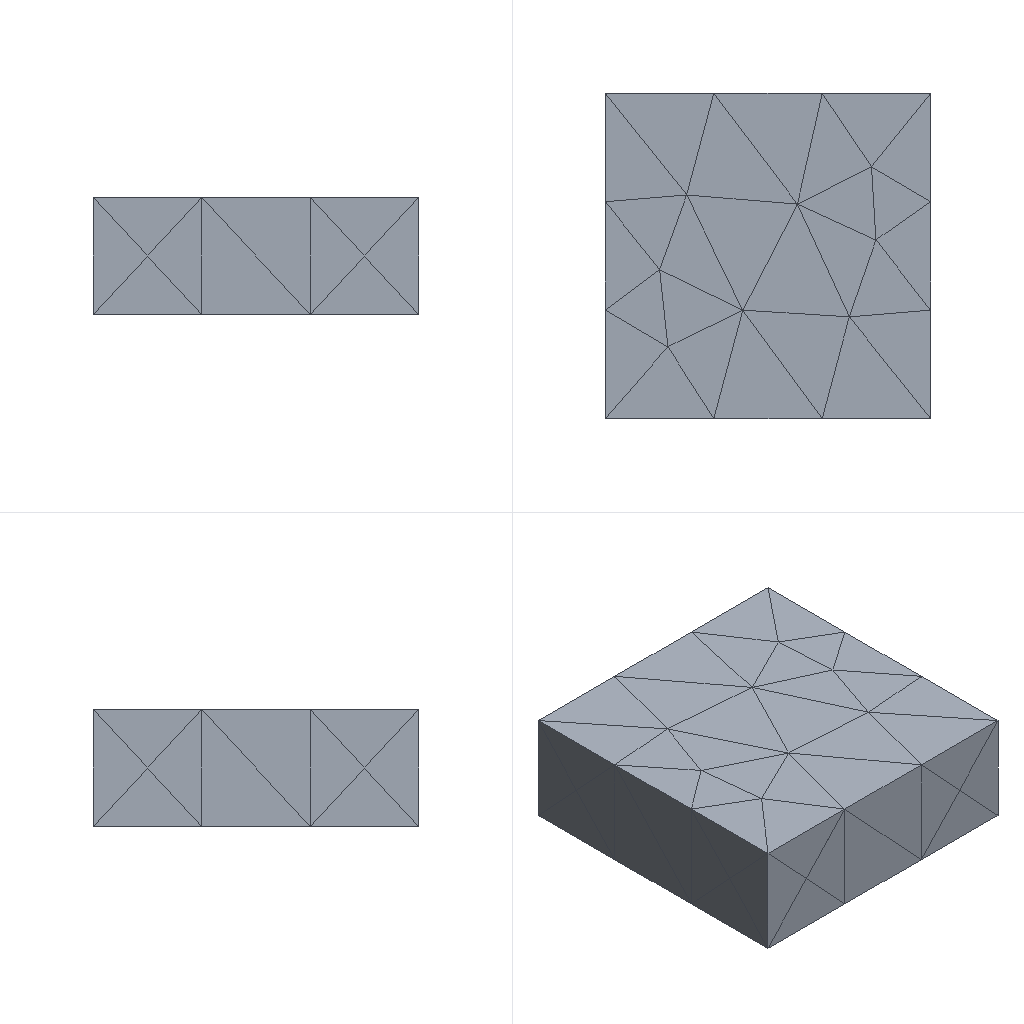Simulation study | ansys mapdl
Set-up summary:
category,name,step,type,value,unit,region
solver,ansys_mapdl
units,mm-N-s-tonne (MPa),,inferred,E=210000 density=
analysis,model,,static
mesh,nodes,,,245
mesh,elements,,,105
element_type,SOLID187,,,105
material,mat 1,,E,210000
material,mat 1,,nu,0.3
load,,model,body load temp,,,all
load,,model,force,"1000 [dir=(0, 0, -1) n=95]",,node list
bc,,model,fixed,"[dofs=UX,UY,UZ n=333]",,node list
Ansys APDL input file, long lists of numbers shortened:
/COM,ANSYS RELEASE 2026 R1           BUILD 26.1      UP20260202       09:09:04
/PREP7
/NOPR
/TITLE,2
ANTYPE, 0
*IF,_CDRDOFF,EQ,1,THEN     !if solid model was read in
_CDRDOFF=             !reset flag, numoffs already performed
*ELSE              !offset database for the following FE model
NUMOFF,NODE,      245
NUMOFF,ELEM,      105
NUMOFF,MAT ,        1
NUMOFF,TYPE,        1
*ENDIF
*SET,_RETURN ,  0.
*SET,_STATUS ,  0.
*SET,_UIQR   ,  95.
*SET,__FLOATPARAMETER__,  245.
DOF,DELETE
ETBLOCK,        1,        1
(2i9,19a9)
        1      187        0        0        0        0        0        0        0        0        0        0        0        0        0        0        0        0        0        0        0
       -1
NBLOCK,6,SOLID,       245,       245
(3i9,6e21.13e3)
        1        0        0 0.0000000000000E+000 2.8000000000000E+001 7.5000000000000E+001
! (244 more lines like these left out)
N,UNBL,LOC,       -1,
EBLOCK,19,SOLID,       105,       105
(19i10)
         1         1         1         1         0         0         0         0        10         0         1       182        56       140       124       184       185       186       187
! (209 more lines like these left out)
        -1
MPTEMP,UNBL, 1, 1,  0.    ,
MPDATA,UNBL, 1,EX  ,       1, 1,  210000.000    ,
MPTEMP,UNBL, 1, 1,  0.    ,
MPDATA,UNBL, 1,NUXY,       1, 1, 0.3    ,
MPTEMP,UNBL, 1, 1,  0.    ,
MPDATA,UNBL, 1,PRXY,       1, 1, 0.3    ,
EXTOPT,ATTR,      0,      0,      0
EXTOPT,ESIZE,  0,  0.
EXTOPT,ACLEAR,      0
TREF,  0.
IRLF,  0
BFUNIF,TEMP,_TINY
ACEL,  0.    ,  0.    ,  0.
OMEGA,  0.    ,  0.    ,  0.
DOMEGA,  0.    ,  0.    ,  0.
CGLOC,  0.    ,  0.    ,  0.
CGOMEGA,  0.    ,  0.    ,  0.
DCGOMG,  0.    ,  0.    ,  0.
KUSE,     0
TIME,  0.
ALPHAD,  0.
BETAD,  0.
DMPRAT,  0.
DMPSTR,  0.
CRPLIM, 0.1    ,   0
CRPLIM,  0.    ,   1
NCNV,     0, 1.000000000E+12,     0,  0.    ,  0.
NEQIT,     0
ERESX,DEFA
DBLOCK,       333
(i9,a6,2(pg16.9))
        1  UX    0.00000000      0.00000000
! (332 more lines like these left out)
       -1
FBLOCK,        95
(i9,a6,2(pg16.9))
       62  FZ   -10.5263158      0.00000000
! (94 more lines like these left out)
       -1
/GO
FINISH
Results summary:
result,analysis_type_db,,,static,unstated
result,n_sets,,,1,unstated
result,load_steps[0].set,load_step=1,,1,unstated
result,load_steps[0].substep,load_step=1,,1,unstated
result,load_steps[0].time,load_step=1,,1,unstated
result,load_steps[0].freq,load_step=1,,1,unstated
result,load_steps[0].max_usum,load_step=1,,0.0001782,unstated
result,load_steps[0].max_seqv,load_step=1,,4.882,unstated
result,load_steps[0].reaction_sum.FX,load_step=1,,3.9142e-12,unstated
result,load_steps[0].reaction_sum.FY,load_step=1,,2.12275e-13,unstated
result,load_steps[0].reaction_sum.FZ,load_step=1,,1000,unstated
result,load_steps[0].reaction_sum.MX,load_step=1,,0,unstated
result,load_steps[0].reaction_sum.MY,load_step=1,,0,unstated
result,load_steps[0].reaction_sum.MZ,load_step=1,,0,unstated
result,convergence,,,results present for all listed sets,unstated